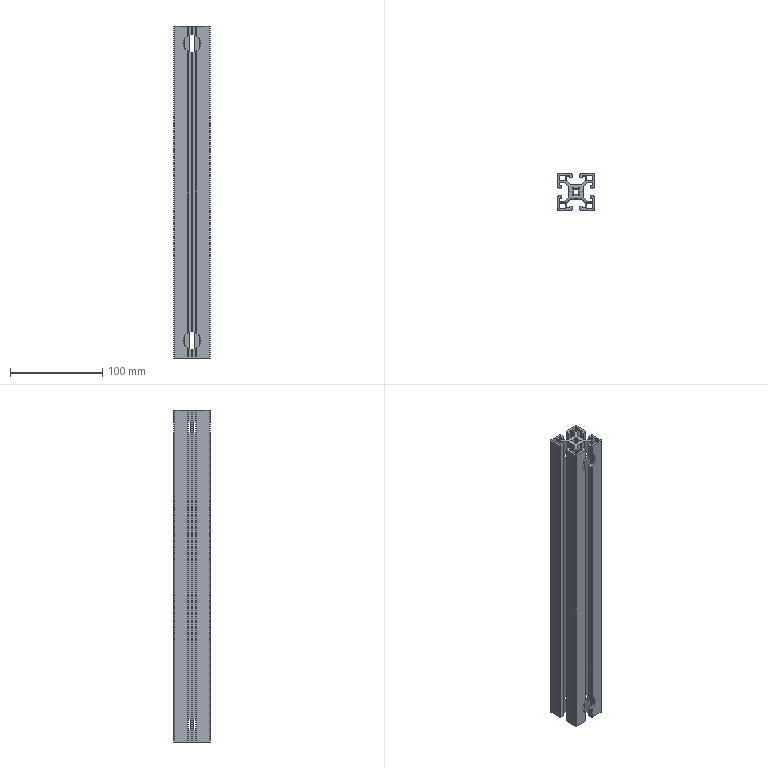Part | NX | features BREP 1 | 1 solid | 273 faces | box 40 x 40 x 360 mm | volume 211725 mm3 | plane 186 | cylinder 87 | commonest cylinder face diameters 1.5 x18 0.6 x16 2 x16 19 x16 6.8 x9 1 x8